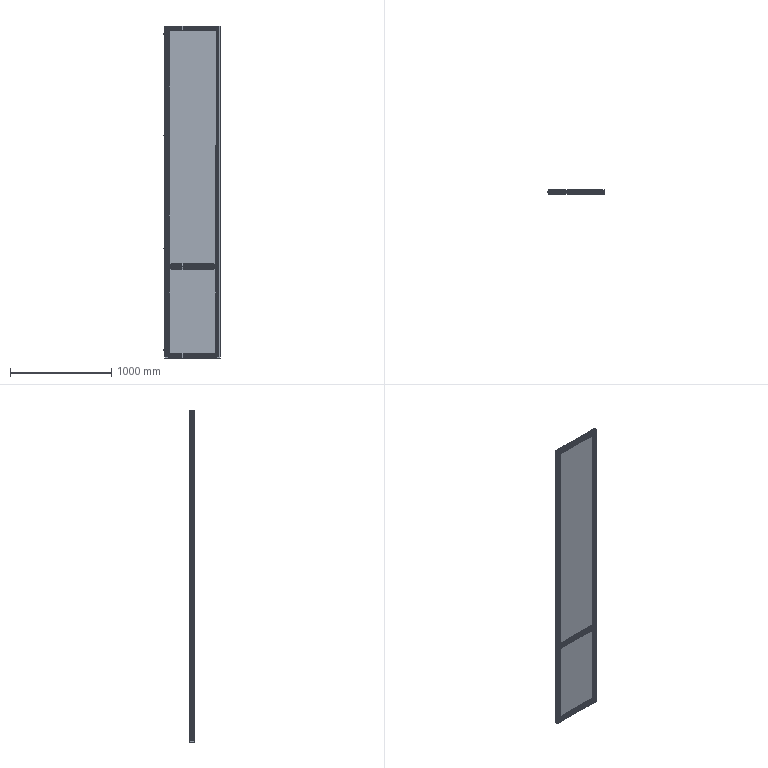Part | SolidWorks | features ReferencePattern 12, LocalLPattern 4 | 31 solids | 1970 faces | box 562.4 x 40 x 3280 mm | volume 12898463 mm3 | plane 1295 | cylinder 623 | cone 44 | spline 8 | commonest cylinder face diameters 5 x104 6.8 x103 2 x54 19 x36 6.6 x32 11 x32